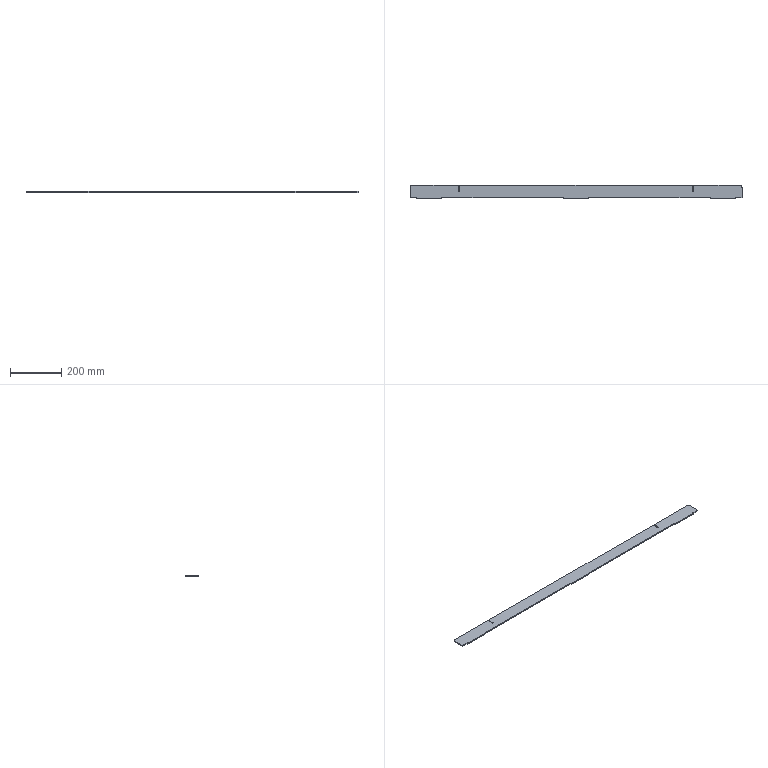Part | SolidWorks | features FlatPattern 1, SMBaseFlange 1, SheetMetal 1 | 1 solid | 28 faces | box 1300 x 54 x 4.5 mm | volume 296674 mm3 | plane 26 | cylinder 2 | commonest cylinder face diameters 20 x2
STEP:
#1=CARTESIAN_POINT('',(713.667,-1108.071,0.));
#2=VERTEX_POINT('',#1);
#3=CARTESIAN_POINT('',(713.667,-1068.071,0.));
#4=VERTEX_POINT('',#3);
#5=CARTESIAN_POINT('',(713.667,-1108.071,0.));
#6=DIRECTION('',(0.,1.,0.));
#7=VECTOR('',#6,1000.);
#8=LINE('',#5,#7);
#9=EDGE_CURVE('',#2,#4,#8,.T.);
#10=ORIENTED_EDGE('',*,*,#9,.F.);
#11=CARTESIAN_POINT('',(713.667,-1108.071,-4.5));
#12=VERTEX_POINT('',#11);
#13=CARTESIAN_POINT('',(713.667,-1108.071,-4.5));
#14=DIRECTION('',(0.,0.,1.));
#15=VECTOR('',#14,1000.);
#16=LINE('',#13,#15);
#17=EDGE_CURVE('',#12,#2,#16,.T.);
#18=ORIENTED_EDGE('',*,*,#17,.F.);
#19=CARTESIAN_POINT('',(713.667,-1068.071,-4.5));
#20=VERTEX_POINT('',#19);
#21=CARTESIAN_POINT('',(713.667,-1108.071,-4.5));
#22=DIRECTION('',(0.,1.,0.));
#23=VECTOR('',#22,1000.);
#24=LINE('',#21,#23);
#25=EDGE_CURVE('',#12,#20,#24,.T.);
#26=ORIENTED_EDGE('',*,*,#25,.T.);
#27=CARTESIAN_POINT('',(713.667,-1068.071,-4.5));
#28=DIRECTION('',(0.,0.,1.));
#29=VECTOR('',#28,1000.);
#30=LINE('',#27,#29);
#31=EDGE_CURVE('',#20,#4,#30,.T.);
#32=ORIENTED_EDGE('',*,*,#31,.T.);
#33=EDGE_LOOP('',(#10,#18,#26,#32));
#34=FACE_OUTER_BOUND('',#33,.T.);
#35=CARTESIAN_POINT('',(713.667,-1108.071,-4.5));
#36=DIRECTION('',(1.,0.,0.));
#37=DIRECTION('',(0.,0.,-1.));
#38=AXIS2_PLACEMENT_3D('',#35,#36,#37);
#39=PLANE('',#38);
#40=ADVANCED_FACE('',(#34),#39,.T.);
#41=CARTESIAN_POINT('',(688.667,-1108.071,0.));
#42=VERTEX_POINT('',#41);
#43=CARTESIAN_POINT('',(713.667,-1108.071,0.));
#44=DIRECTION('',(1.,0.,0.));
#45=VECTOR('',#44,1000.);
#46=LINE('',#43,#45);
#47=EDGE_CURVE('',#42,#2,#46,.T.);
#48=ORIENTED_EDGE('',*,*,#47,.F.);
#49=CARTESIAN_POINT('',(688.667,-1108.071,-4.5));
#50=VERTEX_POINT('',#49);
#51=CARTESIAN_POINT('',(688.667,-1108.071,-4.5));
#52=DIRECTION('',(0.,0.,1.));
#53=VECTOR('',#52,1000.);
#54=LINE('',#51,#53);
#55=EDGE_CURVE('',#50,#42,#54,.T.);
#56=ORIENTED_EDGE('',*,*,#55,.F.);
#57=CARTESIAN_POINT('',(713.667,-1108.071,-4.5));
#58=DIRECTION('',(1.,0.,0.));
#59=VECTOR('',#58,1000.);
#60=LINE('',#57,#59);
#61=EDGE_CURVE('',#50,#12,#60,.T.);
#62=ORIENTED_EDGE('',*,*,#61,.T.);
#63=ORIENTED_EDGE('',*,*,#17,.T.);
#64=EDGE_LOOP('',(#48,#56,#62,#63));
#65=FACE_OUTER_BOUND('',#64,.T.);
#66=CARTESIAN_POINT('',(713.667,-1108.071,-4.5));
#67=DIRECTION('',(0.,-1.,0.));
#68=DIRECTION('',(0.,0.,-1.));
#69=AXIS2_PLACEMENT_3D('',#66,#67,#68);
#70=PLANE('',#69);
#71=ADVANCED_FACE('',(#65),#70,.T.);
#72=CARTESIAN_POINT('',(688.667,-1112.071,0.));
#73=VERTEX_POINT('',#72);
#74=CARTESIAN_POINT('',(688.667,-1108.071,0.));
#75=DIRECTION('',(0.,1.,0.));
#76=VECTOR('',#75,1000.);
#77=LINE('',#74,#76);
#78=EDGE_CURVE('',#73,#42,#77,.T.);
#79=ORIENTED_EDGE('',*,*,#78,.F.);
#80=CARTESIAN_POINT('',(688.667,-1112.071,-4.5));
#81=VERTEX_POINT('',#80);
#82=CARTESIAN_POINT('',(688.667,-1112.071,-4.5));
#83=DIRECTION('',(0.,0.,1.));
#84=VECTOR('',#83,1000.);
#85=LINE('',#82,#84);
#86=EDGE_CURVE('',#81,#73,#85,.T.);
#87=ORIENTED_EDGE('',*,*,#86,.F.);
#88=CARTESIAN_POINT('',(688.667,-1108.071,-4.5));
#89=DIRECTION('',(0.,1.,0.));
#90=VECTOR('',#89,1000.);
#91=LINE('',#88,#90);
#92=EDGE_CURVE('',#81,#50,#91,.T.);
#93=ORIENTED_EDGE('',*,*,#92,.T.);
#94=ORIENTED_EDGE('',*,*,#55,.T.);
#95=EDGE_LOOP('',(#79,#87,#93,#94));
#96=FACE_OUTER_BOUND('',#95,.T.);
#97=CARTESIAN_POINT('',(688.667,-1108.071,-4.5));
#98=DIRECTION('',(1.,0.,0.));
#99=DIRECTION('',(0.,0.,-1.));
#100=AXIS2_PLACEMENT_3D('',#97,#98,#99);
#101=PLANE('',#100);
#102=ADVANCED_FACE('',(#96),#101,.T.);
#103=CARTESIAN_POINT('',(588.667,-1112.071,0.));
#104=VERTEX_POINT('',#103);
#105=CARTESIAN_POINT('',(688.667,-1112.071,0.));
#106=DIRECTION('',(1.,0.,0.));
#107=VECTOR('',#106,1000.);
#108=LINE('',#105,#107);
#109=EDGE_CURVE('',#104,#73,#108,.T.);
#110=ORIENTED_EDGE('',*,*,#109,.F.);
#111=CARTESIAN_POINT('',(588.667,-1112.071,-4.5));
#112=VERTEX_POINT('',#111);
#113=CARTESIAN_POINT('',(588.667,-1112.071,-4.5));
#114=DIRECTION('',(0.,0.,1.));
#115=VECTOR('',#114,1000.);
#116=LINE('',#113,#115);
#117=EDGE_CURVE('',#112,#104,#116,.T.);
#118=ORIENTED_EDGE('',*,*,#117,.F.);
#119=CARTESIAN_POINT('',(688.667,-1112.071,-4.5));
#120=DIRECTION('',(1.,0.,0.));
#121=VECTOR('',#120,1000.);
#122=LINE('',#119,#121);
#123=EDGE_CURVE('',#112,#81,#122,.T.);
#124=ORIENTED_EDGE('',*,*,#123,.T.);
#125=ORIENTED_EDGE('',*,*,#86,.T.);
#126=EDGE_LOOP('',(#110,#118,#124,#125));
#127=FACE_OUTER_BOUND('',#126,.T.);
#128=CARTESIAN_POINT('',(688.667,-1112.071,-4.5));
#129=DIRECTION('',(0.,-1.,0.));
#130=DIRECTION('',(0.,0.,-1.));
#131=AXIS2_PLACEMENT_3D('',#128,#129,#130);
#132=PLANE('',#131);
#133=ADVANCED_FACE('',(#127),#132,.T.);
#134=CARTESIAN_POINT('',(588.667,-1108.071,0.));
#135=VERTEX_POINT('',#134);
#136=CARTESIAN_POINT('',(588.667,-1112.071,0.));
#137=DIRECTION('',(0.,-1.,0.));
#138=VECTOR('',#137,1000.);
#139=LINE('',#136,#138);
#140=EDGE_CURVE('',#135,#104,#139,.T.);
#141=ORIENTED_EDGE('',*,*,#140,.F.);
#142=CARTESIAN_POINT('',(588.667,-1108.071,-4.5));
#143=VERTEX_POINT('',#142);
#144=CARTESIAN_POINT('',(588.667,-1108.071,-4.5));
#145=DIRECTION('',(0.,0.,1.));
#146=VECTOR('',#145,1000.);
#147=LINE('',#144,#146);
#148=EDGE_CURVE('',#143,#135,#147,.T.);
#149=ORIENTED_EDGE('',*,*,#148,.F.);
#150=CARTESIAN_POINT('',(588.667,-1112.071,-4.5));
#151=DIRECTION('',(0.,-1.,0.));
#152=VECTOR('',#151,1000.);
#153=LINE('',#150,#152);
#154=EDGE_CURVE('',#143,#112,#153,.T.);
#155=ORIENTED_EDGE('',*,*,#154,.T.);
#156=ORIENTED_EDGE('',*,*,#117,.T.);
#157=EDGE_LOOP('',(#141,#149,#155,#156));
#158=FACE_OUTER_BOUND('',#157,.T.);
#159=CARTESIAN_POINT('',(588.667,-1112.071,-4.5));
#160=DIRECTION('',(-1.,0.,0.));
#161=DIRECTION('',(0.,0.,1.));
#162=AXIS2_PLACEMENT_3D('',#159,#160,#161);
#163=PLANE('',#162);
#164=ADVANCED_FACE('',(#158),#163,.T.);
#165=CARTESIAN_POINT('',(113.667,-1108.071,0.));
#166=VERTEX_POINT('',#165);
#167=CARTESIAN_POINT('',(588.667,-1108.071,0.));
#168=DIRECTION('',(1.,0.,0.));
#169=VECTOR('',#168,1000.);
#170=LINE('',#167,#169);
#171=EDGE_CURVE('',#166,#135,#170,.T.);
#172=ORIENTED_EDGE('',*,*,#171,.F.);
#173=CARTESIAN_POINT('',(113.667,-1108.071,-4.5));
#174=VERTEX_POINT('',#173);
#175=CARTESIAN_POINT('',(113.667,-1108.071,-4.5));
#176=DIRECTION('',(0.,0.,1.));
#177=VECTOR('',#176,1000.);
#178=LINE('',#175,#177);
#179=EDGE_CURVE('',#174,#166,#178,.T.);
#180=ORIENTED_EDGE('',*,*,#179,.F.);
#181=CARTESIAN_POINT('',(588.667,-1108.071,-4.5));
#182=DIRECTION('',(1.,0.,0.));
#183=VECTOR('',#182,1000.);
#184=LINE('',#181,#183);
#185=EDGE_CURVE('',#174,#143,#184,.T.);
#186=ORIENTED_EDGE('',*,*,#185,.T.);
#187=ORIENTED_EDGE('',*,*,#148,.T.);
#188=EDGE_LOOP('',(#172,#180,#186,#187));
#189=FACE_OUTER_BOUND('',#188,.T.);
#190=CARTESIAN_POINT('',(588.667,-1108.071,-4.5));
#191=DIRECTION('',(0.,-1.,0.));
#192=DIRECTION('',(0.,0.,-1.));
#193=AXIS2_PLACEMENT_3D('',#190,#191,#192);
#194=PLANE('',#193);
#195=ADVANCED_FACE('',(#189),#194,.T.);
#196=CARTESIAN_POINT('',(113.667,-1112.071,0.));
#197=VERTEX_POINT('',#196);
#198=CARTESIAN_POINT('',(113.667,-1108.071,0.));
#199=DIRECTION('',(0.,1.,0.));
#200=VECTOR('',#199,1000.);
#201=LINE('',#198,#200);
#202=EDGE_CURVE('',#197,#166,#201,.T.);
#203=ORIENTED_EDGE('',*,*,#202,.F.);
#204=CARTESIAN_POINT('',(113.667,-1112.071,-4.5));
#205=VERTEX_POINT('',#204);
#206=CARTESIAN_POINT('',(113.667,-1112.071,-4.5));
#207=DIRECTION('',(0.,0.,1.));
#208=VECTOR('',#207,1000.);
#209=LINE('',#206,#208);
#210=EDGE_CURVE('',#205,#197,#209,.T.);
#211=ORIENTED_EDGE('',*,*,#210,.F.);
#212=CARTESIAN_POINT('',(113.667,-1108.071,-4.5));
#213=DIRECTION('',(0.,1.,0.));
#214=VECTOR('',#213,1000.);
#215=LINE('',#212,#214);
#216=EDGE_CURVE('',#205,#174,#215,.T.);
#217=ORIENTED_EDGE('',*,*,#216,.T.);
#218=ORIENTED_EDGE('',*,*,#179,.T.);
#219=EDGE_LOOP('',(#203,#211,#217,#218));
#220=FACE_OUTER_BOUND('',#219,.T.);
#221=CARTESIAN_POINT('',(113.667,-1108.071,-4.5));
#222=DIRECTION('',(1.,0.,0.));
#223=DIRECTION('',(0.,1.,0.));
#224=AXIS2_PLACEMENT_3D('',#221,#222,#223);
#225=PLANE('',#224);
#226=ADVANCED_FACE('',(#220),#225,.T.);
#227=CARTESIAN_POINT('',(13.667,-1112.071,0.));
#228=VERTEX_POINT('',#227);
#229=CARTESIAN_POINT('',(113.667,-1112.071,0.));
#230=DIRECTION('',(1.,0.,0.));
#231=VECTOR('',#230,1000.);
#232=LINE('',#229,#231);
#233=EDGE_CURVE('',#228,#197,#232,.T.);
#234=ORIENTED_EDGE('',*,*,#233,.F.);
#235=CARTESIAN_POINT('',(13.667,-1112.071,-4.5));
#236=VERTEX_POINT('',#235);
#237=CARTESIAN_POINT('',(13.667,-1112.071,-4.5));
#238=DIRECTION('',(0.,0.,1.));
#239=VECTOR('',#238,1000.);
#240=LINE('',#237,#239);
#241=EDGE_CURVE('',#236,#228,#240,.T.);
#242=ORIENTED_EDGE('',*,*,#241,.F.);
#243=CARTESIAN_POINT('',(113.667,-1112.071,-4.5));
#244=DIRECTION('',(1.,0.,0.));
#245=VECTOR('',#244,1000.);
#246=LINE('',#243,#245);
#247=EDGE_CURVE('',#236,#205,#246,.T.);
#248=ORIENTED_EDGE('',*,*,#247,.T.);
#249=ORIENTED_EDGE('',*,*,#210,.T.);
#250=EDGE_LOOP('',(#234,#242,#248,#249));
#251=FACE_OUTER_BOUND('',#250,.T.);
#252=CARTESIAN_POINT('',(113.667,-1112.071,-4.5));
#253=DIRECTION('',(0.,-1.,0.));
#254=DIRECTION('',(0.,0.,-1.));
#255=AXIS2_PLACEMENT_3D('',#252,#253,#254);
#256=PLANE('',#255);
#257=ADVANCED_FACE('',(#251),#256,.T.);
#258=CARTESIAN_POINT('',(13.667,-1108.071,0.));
#259=VERTEX_POINT('',#258);
#260=CARTESIAN_POINT('',(13.667,-1112.071,0.));
#261=DIRECTION('',(0.,-1.,0.));
#262=VECTOR('',#261,1000.);
#263=LINE('',#260,#262);
#264=EDGE_CURVE('',#259,#228,#263,.T.);
#265=ORIENTED_EDGE('',*,*,#264,.F.);
#266=CARTESIAN_POINT('',(13.667,-1108.071,-4.5));
#267=VERTEX_POINT('',#266);
#268=CARTESIAN_POINT('',(13.667,-1108.071,-4.5));
#269=DIRECTION('',(0.,0.,1.));
#270=VECTOR('',#269,1000.);
#271=LINE('',#268,#270);
#272=EDGE_CURVE('',#267,#259,#271,.T.);
#273=ORIENTED_EDGE('',*,*,#272,.F.);
#274=CARTESIAN_POINT('',(13.667,-1112.071,-4.5));
#275=DIRECTION('',(0.,-1.,0.));
#276=VECTOR('',#275,1000.);
#277=LINE('',#274,#276);
#278=EDGE_CURVE('',#267,#236,#277,.T.);
#279=ORIENTED_EDGE('',*,*,#278,.T.);
#280=ORIENTED_EDGE('',*,*,#241,.T.);
#281=EDGE_LOOP('',(#265,#273,#279,#280));
#282=FACE_OUTER_BOUND('',#281,.T.);
#283=CARTESIAN_POINT('',(13.667,-1112.071,-4.5));
#284=DIRECTION('',(-1.,0.,0.));
#285=DIRECTION('',(0.,-1.,0.));
#286=AXIS2_PLACEMENT_3D('',#283,#284,#285);
#287=PLANE('',#286);
#288=ADVANCED_FACE('',(#282),#287,.T.);
#289=CARTESIAN_POINT('',(-461.333,-1108.071,0.));
#290=VERTEX_POINT('',#289);
#291=CARTESIAN_POINT('',(13.667,-1108.071,0.));
#292=DIRECTION('',(1.,0.,0.));
#293=VECTOR('',#292,1000.);
#294=LINE('',#291,#293);
#295=EDGE_CURVE('',#290,#259,#294,.T.);
#296=ORIENTED_EDGE('',*,*,#295,.F.);
#297=CARTESIAN_POINT('',(-461.333,-1108.071,-4.5));
#298=VERTEX_POINT('',#297);
#299=CARTESIAN_POINT('',(-461.333,-1108.071,-4.5));
#300=DIRECTION('',(0.,0.,1.));
#301=VECTOR('',#300,1000.);
#302=LINE('',#299,#301);
#303=EDGE_CURVE('',#298,#290,#302,.T.);
#304=ORIENTED_EDGE('',*,*,#303,.F.);
#305=CARTESIAN_POINT('',(13.667,-1108.071,-4.5));
#306=DIRECTION('',(1.,0.,0.));
#307=VECTOR('',#306,1000.);
#308=LINE('',#305,#307);
#309=EDGE_CURVE('',#298,#267,#308,.T.);
#310=ORIENTED_EDGE('',*,*,#309,.T.);
#311=ORIENTED_EDGE('',*,*,#272,.T.);
#312=EDGE_LOOP('',(#296,#304,#310,#311));
#313=FACE_OUTER_BOUND('',#312,.T.);
#314=CARTESIAN_POINT('',(13.667,-1108.071,-4.5));
#315=DIRECTION('',(0.,-1.,0.));
#316=DIRECTION('',(0.,0.,-1.));
#317=AXIS2_PLACEMENT_3D('',#314,#315,#316);
#318=PLANE('',#317);
#319=ADVANCED_FACE('',(#313),#318,.T.);
#320=CARTESIAN_POINT('',(-461.333,-1112.071,0.));
#321=VERTEX_POINT('',#320);
#322=CARTESIAN_POINT('',(-461.333,-1112.071,0.));
#323=DIRECTION('',(0.,1.,0.));
#324=VECTOR('',#323,1000.);
#325=LINE('',#322,#324);
#326=EDGE_CURVE('',#321,#290,#325,.T.);
#327=ORIENTED_EDGE('',*,*,#326,.F.);
#328=CARTESIAN_POINT('',(-461.333,-1112.071,-4.5));
#329=VERTEX_POINT('',#328);
#330=CARTESIAN_POINT('',(-461.333,-1112.071,-4.5));
#331=DIRECTION('',(0.,0.,1.));
#332=VECTOR('',#331,1000.);
#333=LINE('',#330,#332);
#334=EDGE_CURVE('',#329,#321,#333,.T.);
#335=ORIENTED_EDGE('',*,*,#334,.F.);
#336=CARTESIAN_POINT('',(-461.333,-1112.071,-4.5));
#337=DIRECTION('',(0.,1.,0.));
#338=VECTOR('',#337,1000.);
#339=LINE('',#336,#338);
#340=EDGE_CURVE('',#329,#298,#339,.T.);
#341=ORIENTED_EDGE('',*,*,#340,.T.);
#342=ORIENTED_EDGE('',*,*,#303,.T.);
#343=EDGE_LOOP('',(#327,#335,#341,#342));
#344=FACE_OUTER_BOUND('',#343,.T.);
#345=CARTESIAN_POINT('',(-461.333,-1112.071,-4.5));
#346=DIRECTION('',(1.,0.,0.));
#347=DIRECTION('',(0.,0.,-1.));
#348=AXIS2_PLACEMENT_3D('',#345,#346,#347);
#349=PLANE('',#348);
#350=ADVANCED_FACE('',(#344),#349,.T.);
#351=CARTESIAN_POINT('',(-561.333,-1112.071,0.));
#352=VERTEX_POINT('',#351);
#353=CARTESIAN_POINT('',(-561.333,-1112.071,0.));
#354=DIRECTION('',(1.,0.,0.));
#355=VECTOR('',#354,1000.);
#356=LINE('',#353,#355);
#357=EDGE_CURVE('',#352,#321,#356,.T.);
#358=ORIENTED_EDGE('',*,*,#357,.F.);
#359=CARTESIAN_POINT('',(-561.333,-1112.071,-4.5));
#360=VERTEX_POINT('',#359);
#361=CARTESIAN_POINT('',(-561.333,-1112.071,-4.5));
#362=DIRECTION('',(0.,0.,1.));
#363=VECTOR('',#362,1000.);
#364=LINE('',#361,#363);
#365=EDGE_CURVE('',#360,#352,#364,.T.);
#366=ORIENTED_EDGE('',*,*,#365,.F.);
#367=CARTESIAN_POINT('',(-561.333,-1112.071,-4.5));
#368=DIRECTION('',(1.,0.,0.));
#369=VECTOR('',#368,1000.);
#370=LINE('',#367,#369);
#371=EDGE_CURVE('',#360,#329,#370,.T.);
#372=ORIENTED_EDGE('',*,*,#371,.T.);
#373=ORIENTED_EDGE('',*,*,#334,.T.);
#374=EDGE_LOOP('',(#358,#366,#372,#373));
#375=FACE_OUTER_BOUND('',#374,.T.);
#376=CARTESIAN_POINT('',(-561.333,-1112.071,-4.5));
#377=DIRECTION('',(0.,-1.,0.));
#378=DIRECTION('',(0.,0.,-1.));
#379=AXIS2_PLACEMENT_3D('',#376,#377,#378);
#380=PLANE('',#379);
#381=ADVANCED_FACE('',(#375),#380,.T.);
#382=CARTESIAN_POINT('',(-561.333,-1108.071,0.));
#383=VERTEX_POINT('',#382);
#384=CARTESIAN_POINT('',(-561.333,-1108.071,0.));
#385=DIRECTION('',(0.,-1.,0.));
#386=VECTOR('',#385,1000.);
#387=LINE('',#384,#386);
#388=EDGE_CURVE('',#383,#352,#387,.T.);
#389=ORIENTED_EDGE('',*,*,#388,.F.);
#390=CARTESIAN_POINT('',(-561.333,-1108.071,-4.5));
#391=VERTEX_POINT('',#390);
#392=CARTESIAN_POINT('',(-561.333,-1108.071,-4.5));
#393=DIRECTION('',(0.,0.,1.));
#394=VECTOR('',#393,1000.);
#395=LINE('',#392,#394);
#396=EDGE_CURVE('',#391,#383,#395,.T.);
#397=ORIENTED_EDGE('',*,*,#396,.F.);
#398=CARTESIAN_POINT('',(-561.333,-1108.071,-4.5));
#399=DIRECTION('',(0.,-1.,0.));
#400=VECTOR('',#399,1000.);
#401=LINE('',#398,#400);
#402=EDGE_CURVE('',#391,#360,#401,.T.);
#403=ORIENTED_EDGE('',*,*,#402,.T.);
#404=ORIENTED_EDGE('',*,*,#365,.T.);
#405=EDGE_LOOP('',(#389,#397,#403,#404));
#406=FACE_OUTER_BOUND('',#405,.T.);
#407=CARTESIAN_POINT('',(-561.333,-1108.071,-4.5));
#408=DIRECTION('',(-1.,0.,0.));
#409=DIRECTION('',(0.,0.,1.));
#410=AXIS2_PLACEMENT_3D('',#407,#408,#409);
#411=PLANE('',#410);
#412=ADVANCED_FACE('',(#406),#411,.T.);
#413=CARTESIAN_POINT('',(-586.333,-1108.071,0.));
#414=VERTEX_POINT('',#413);
#415=CARTESIAN_POINT('',(-561.333,-1108.071,0.));
#416=DIRECTION('',(1.,0.,0.));
#417=VECTOR('',#416,1000.);
#418=LINE('',#415,#417);
#419=EDGE_CURVE('',#414,#383,#418,.T.);
#420=ORIENTED_EDGE('',*,*,#419,.F.);
#421=CARTESIAN_POINT('',(-586.333,-1108.071,-4.5));
#422=VERTEX_POINT('',#421);
#423=CARTESIAN_POINT('',(-586.333,-1108.071,-4.5));
#424=DIRECTION('',(0.,0.,1.));
#425=VECTOR('',#424,1000.);
#426=LINE('',#423,#425);
#427=EDGE_CURVE('',#422,#414,#426,.T.);
#428=ORIENTED_EDGE('',*,*,#427,.F.);
#429=CARTESIAN_POINT('',(-561.333,-1108.071,-4.5));
#430=DIRECTION('',(1.,0.,0.));
#431=VECTOR('',#430,1000.);
#432=LINE('',#429,#431);
#433=EDGE_CURVE('',#422,#391,#432,.T.);
#434=ORIENTED_EDGE('',*,*,#433,.T.);
#435=ORIENTED_EDGE('',*,*,#396,.T.);
#436=EDGE_LOOP('',(#420,#428,#434,#435));
#437=FACE_OUTER_BOUND('',#436,.T.);
#438=CARTESIAN_POINT('',(-561.333,-1108.071,-4.5));
#439=DIRECTION('',(0.,-1.,0.));
#440=DIRECTION('',(0.,0.,-1.));
#441=AXIS2_PLACEMENT_3D('',#438,#439,#440);
#442=PLANE('',#441);
#443=ADVANCED_FACE('',(#437),#442,.T.);
#444=CARTESIAN_POINT('',(-586.333,-1068.071,0.));
#445=VERTEX_POINT('',#444);
#446=CARTESIAN_POINT('',(-586.333,-1108.071,0.));
#447=DIRECTION('',(0.,-1.,0.));
#448=VECTOR('',#447,1000.);
#449=LINE('',#446,#448);
#450=EDGE_CURVE('',#445,#414,#449,.T.);
#451=ORIENTED_EDGE('',*,*,#450,.F.);
#452=CARTESIAN_POINT('',(-586.333,-1068.071,-4.5));
#453=VERTEX_POINT('',#452);
#454=CARTESIAN_POINT('',(-586.333,-1068.071,-4.5));
#455=DIRECTION('',(0.,0.,1.));
#456=VECTOR('',#455,1000.);
#457=LINE('',#454,#456);
#458=EDGE_CURVE('',#453,#445,#457,.T.);
#459=ORIENTED_EDGE('',*,*,#458,.F.);
#460=CARTESIAN_POINT('',(-586.333,-1108.071,-4.5));
#461=DIRECTION('',(0.,-1.,0.));
#462=VECTOR('',#461,1000.);
#463=LINE('',#460,#462);
#464=EDGE_CURVE('',#453,#422,#463,.T.);
#465=ORIENTED_EDGE('',*,*,#464,.T.);
#466=ORIENTED_EDGE('',*,*,#427,.T.);
#467=EDGE_LOOP('',(#451,#459,#465,#466));
#468=FACE_OUTER_BOUND('',#467,.T.);
#469=CARTESIAN_POINT('',(-586.333,-1108.071,-4.5));
#470=DIRECTION('',(-1.,0.,0.));
#471=DIRECTION('',(0.,0.,1.));
#472=AXIS2_PLACEMENT_3D('',#469,#470,#471);
#473=PLANE('',#472);
#474=ADVANCED_FACE('',(#468),#473,.T.);
#475=CARTESIAN_POINT('',(-576.333,-1058.071,0.));
#476=VERTEX_POINT('',#475);
#477=CARTESIAN_POINT('',(-576.333,-1068.071,0.));
#478=DIRECTION('',(0.,0.,1.));
#479=DIRECTION('',(1.,0.,0.));
#480=AXIS2_PLACEMENT_3D('',#477,#478,#479);
#481=CIRCLE('',#480,10.);
#482=EDGE_CURVE('',#476,#445,#481,.T.);
#483=ORIENTED_EDGE('',*,*,#482,.F.);
#484=CARTESIAN_POINT('',(-576.333,-1058.071,-4.5));
#485=VERTEX_POINT('',#484);
#486=CARTESIAN_POINT('',(-576.333,-1058.071,-4.5));
#487=DIRECTION('',(0.,0.,1.));
#488=VECTOR('',#487,1000.);
#489=LINE('',#486,#488);
#490=EDGE_CURVE('',#485,#476,#489,.T.);
#491=ORIENTED_EDGE('',*,*,#490,.F.);
#492=CARTESIAN_POINT('',(-576.333,-1068.071,-4.5));
#493=DIRECTION('',(0.,0.,1.));
#494=DIRECTION('',(1.,0.,0.));
#495=AXIS2_PLACEMENT_3D('',#492,#493,#494);
#496=CIRCLE('',#495,10.);
#497=EDGE_CURVE('',#485,#453,#496,.T.);
#498=ORIENTED_EDGE('',*,*,#497,.T.);
#499=ORIENTED_EDGE('',*,*,#458,.T.);
#500=EDGE_LOOP('',(#483,#491,#498,#499));
#501=FACE_OUTER_BOUND('',#500,.T.);
#502=CARTESIAN_POINT('',(-576.333,-1068.071,-4.5));
#503=DIRECTION('',(0.,0.,1.));
#504=DIRECTION('',(1.,0.,0.));
#505=AXIS2_PLACEMENT_3D('',#502,#503,#504);
#506=CYLINDRICAL_SURFACE('',#505,10.);
#507=ADVANCED_FACE('',(#501),#506,.T.);
#508=CARTESIAN_POINT('',(-396.333,-1058.071,0.));
#509=VERTEX_POINT('',#508);
#510=CARTESIAN_POINT('',(-396.333,-1058.071,0.));
#511=DIRECTION('',(-1.,0.,0.));
#512=VECTOR('',#511,1000.);
#513=LINE('',#510,#512);
#514=EDGE_CURVE('',#509,#476,#513,.T.);
#515=ORIENTED_EDGE('',*,*,#514,.F.);
#516=CARTESIAN_POINT('',(-396.333,-1058.071,-4.5));
#517=VERTEX_POINT('',#516);
#518=CARTESIAN_POINT('',(-396.333,-1058.071,-4.5));
#519=DIRECTION('',(0.,0.,1.));
#520=VECTOR('',#519,1000.);
#521=LINE('',#518,#520);
#522=EDGE_CURVE('',#517,#509,#521,.T.);
#523=ORIENTED_EDGE('',*,*,#522,.F.);
#524=CARTESIAN_POINT('',(-396.333,-1058.071,-4.5));
#525=DIRECTION('',(-1.,0.,0.));
#526=VECTOR('',#525,1000.);
#527=LINE('',#524,#526);
#528=EDGE_CURVE('',#517,#485,#527,.T.);
#529=ORIENTED_EDGE('',*,*,#528,.T.);
#530=ORIENTED_EDGE('',*,*,#490,.T.);
#531=EDGE_LOOP('',(#515,#523,#529,#530));
#532=FACE_OUTER_BOUND('',#531,.T.);
#533=CARTESIAN_POINT('',(-396.333,-1058.071,-4.5));
#534=DIRECTION('',(0.,1.,0.));
#535=DIRECTION('',(0.,0.,1.));
#536=AXIS2_PLACEMENT_3D('',#533,#534,#535);
#537=PLANE('',#536);
#538=ADVANCED_FACE('',(#532),#537,.T.);
#539=CARTESIAN_POINT('',(-396.333,-1083.571,0.));
#540=VERTEX_POINT('',#539);
#541=CARTESIAN_POINT('',(-396.333,-1083.571,0.));
#542=DIRECTION('',(0.,1.,0.));
#543=VECTOR('',#542,1000.);
#544=LINE('',#541,#543);
#545=EDGE_CURVE('',#540,#509,#544,.T.);
#546=ORIENTED_EDGE('',*,*,#545,.F.);
#547=CARTESIAN_POINT('',(-396.333,-1083.571,-4.5));
#548=VERTEX_POINT('',#547);
#549=CARTESIAN_POINT('',(-396.333,-1083.571,-4.5));
#550=DIRECTION('',(0.,0.,1.));
#551=VECTOR('',#550,1000.);
#552=LINE('',#549,#551);
#553=EDGE_CURVE('',#548,#540,#552,.T.);
#554=ORIENTED_EDGE('',*,*,#553,.F.);
#555=CARTESIAN_POINT('',(-396.333,-1083.571,-4.5));
#556=DIRECTION('',(0.,1.,0.));
#557=VECTOR('',#556,1000.);
#558=LINE('',#555,#557);
#559=EDGE_CURVE('',#548,#517,#558,.T.);
#560=ORIENTED_EDGE('',*,*,#559,.T.);
#561=ORIENTED_EDGE('',*,*,#522,.T.);
#562=EDGE_LOOP('',(#546,#554,#560,#561));
#563=FACE_OUTER_BOUND('',#562,.T.);
#564=CARTESIAN_POINT('',(-396.333,-1083.571,-4.5));
#565=DIRECTION('',(1.,0.,0.));
#566=DIRECTION('',(0.,0.,-1.));
#567=AXIS2_PLACEMENT_3D('',#564,#565,#566);
#568=PLANE('',#567);
#569=ADVANCED_FACE('',(#563),#568,.T.);
#570=CARTESIAN_POINT('',(-391.833,-1083.571,0.));
#571=VERTEX_POINT('',#570);
#572=CARTESIAN_POINT('',(-391.833,-1083.571,0.));
#573=DIRECTION('',(-1.,0.,0.));
#574=VECTOR('',#573,1000.);
#575=LINE('',#572,#574);
#576=EDGE_CURVE('',#571,#540,#575,.T.);
#577=ORIENTED_EDGE('',*,*,#576,.F.);
#578=CARTESIAN_POINT('',(-391.833,-1083.571,-4.5));
#579=VERTEX_POINT('',#578);
#580=CARTESIAN_POINT('',(-391.833,-1083.571,-4.5));
#581=DIRECTION('',(0.,0.,1.));
#582=VECTOR('',#581,1000.);
#583=LINE('',#580,#582);
#584=EDGE_CURVE('',#579,#571,#583,.T.);
#585=ORIENTED_EDGE('',*,*,#584,.F.);
#586=CARTESIAN_POINT('',(-391.833,-1083.571,-4.5));
#587=DIRECTION('',(-1.,0.,0.));
#588=VECTOR('',#587,1000.);
#589=LINE('',#586,#588);
#590=EDGE_CURVE('',#579,#548,#589,.T.);
#591=ORIENTED_EDGE('',*,*,#590,.T.);
#592=ORIENTED_EDGE('',*,*,#553,.T.);
#593=EDGE_LOOP('',(#577,#585,#591,#592));
#594=FACE_OUTER_BOUND('',#593,.T.);
#595=CARTESIAN_POINT('',(-391.833,-1083.571,-4.5));
#596=DIRECTION('',(0.,1.,0.));
#597=DIRECTION('',(0.,0.,1.));
#598=AXIS2_PLACEMENT_3D('',#595,#596,#597);
#599=PLANE('',#598);
#600=ADVANCED_FACE('',(#594),#599,.T.);
#601=CARTESIAN_POINT('',(-391.833,-1058.071,0.));
#602=VERTEX_POINT('',#601);
#603=CARTESIAN_POINT('',(-391.833,-1058.071,0.));
#604=DIRECTION('',(0.,-1.,0.));
#605=VECTOR('',#604,1000.);
#606=LINE('',#603,#605);
#607=EDGE_CURVE('',#602,#571,#606,.T.);
#608=ORIENTED_EDGE('',*,*,#607,.F.);
#609=CARTESIAN_POINT('',(-391.833,-1058.071,-4.5));
#610=VERTEX_POINT('',#609);
#611=CARTESIAN_POINT('',(-391.833,-1058.071,-4.5));
#612=DIRECTION('',(0.,0.,1.));
#613=VECTOR('',#612,1000.);
#614=LINE('',#611,#613);
#615=EDGE_CURVE('',#610,#602,#614,.T.);
#616=ORIENTED_EDGE('',*,*,#615,.F.);
#617=CARTESIAN_POINT('',(-391.833,-1058.071,-4.5));
#618=DIRECTION('',(0.,-1.,0.));
#619=VECTOR('',#618,1000.);
#620=LINE('',#617,#619);
#621=EDGE_CURVE('',#610,#579,#620,.T.);
#622=ORIENTED_EDGE('',*,*,#621,.T.);
#623=ORIENTED_EDGE('',*,*,#584,.T.);
#624=EDGE_LOOP('',(#608,#616,#622,#623));
#625=FACE_OUTER_BOUND('',#624,.T.);
#626=CARTESIAN_POINT('',(-391.833,-1058.071,-4.5));
#627=DIRECTION('',(-1.,0.,0.));
#628=DIRECTION('',(0.,0.,1.));
#629=AXIS2_PLACEMENT_3D('',#626,#627,#628);
#630=PLANE('',#629);
#631=ADVANCED_FACE('',(#625),#630,.T.);
#632=CARTESIAN_POINT('',(519.167,-1058.071,0.));
#633=VERTEX_POINT('',#632);
#634=CARTESIAN_POINT('',(519.167,-1058.071,0.));
#635=DIRECTION('',(-1.,0.,0.));
#636=VECTOR('',#635,1000.);
#637=LINE('',#634,#636);
#638=EDGE_CURVE('',#633,#602,#637,.T.);
#639=ORIENTED_EDGE('',*,*,#638,.F.);
#640=CARTESIAN_POINT('',(519.167,-1058.071,-4.5));
#641=VERTEX_POINT('',#640);
#642=CARTESIAN_POINT('',(519.167,-1058.071,-4.5));
#643=DIRECTION('',(0.,0.,1.));
#644=VECTOR('',#643,1000.);
#645=LINE('',#642,#644);
#646=EDGE_CURVE('',#641,#633,#645,.T.);
#647=ORIENTED_EDGE('',*,*,#646,.F.);
#648=CARTESIAN_POINT('',(519.167,-1058.071,-4.5));
#649=DIRECTION('',(-1.,0.,0.));
#650=VECTOR('',#649,1000.);
#651=LINE('',#648,#650);
#652=EDGE_CURVE('',#641,#610,#651,.T.);
#653=ORIENTED_EDGE('',*,*,#652,.T.);
#654=ORIENTED_EDGE('',*,*,#615,.T.);
#655=EDGE_LOOP('',(#639,#647,#653,#654));
#656=FACE_OUTER_BOUND('',#655,.T.);
#657=CARTESIAN_POINT('',(519.167,-1058.071,-4.5));
#658=DIRECTION('',(0.,1.,0.));
#659=DIRECTION('',(0.,0.,1.));
#660=AXIS2_PLACEMENT_3D('',#657,#658,#659);
#661=PLANE('',#660);
#662=ADVANCED_FACE('',(#656),#661,.T.);
#663=CARTESIAN_POINT('',(519.167,-1083.571,0.));
#664=VERTEX_POINT('',#663);
#665=CARTESIAN_POINT('',(519.167,-1083.571,0.));
#666=DIRECTION('',(0.,1.,0.));
#667=VECTOR('',#666,1000.);
#668=LINE('',#665,#667);
#669=EDGE_CURVE('',#664,#633,#668,.T.);
#670=ORIENTED_EDGE('',*,*,#669,.F.);
#671=CARTESIAN_POINT('',(519.167,-1083.571,-4.5));
#672=VERTEX_POINT('',#671);
#673=CARTESIAN_POINT('',(519.167,-1083.571,-4.5));
#674=DIRECTION('',(0.,0.,1.));
#675=VECTOR('',#674,1000.);
#676=LINE('',#673,#675);
#677=EDGE_CURVE('',#672,#664,#676,.T.);
#678=ORIENTED_EDGE('',*,*,#677,.F.);
#679=CARTESIAN_POINT('',(519.167,-1083.571,-4.5));
#680=DIRECTION('',(0.,1.,0.));
#681=VECTOR('',#680,1000.);
#682=LINE('',#679,#681);
#683=EDGE_CURVE('',#672,#641,#682,.T.);
#684=ORIENTED_EDGE('',*,*,#683,.T.);
#685=ORIENTED_EDGE('',*,*,#646,.T.);
#686=EDGE_LOOP('',(#670,#678,#684,#685));
#687=FACE_OUTER_BOUND('',#686,.T.);
#688=CARTESIAN_POINT('',(519.167,-1083.571,-4.5));
#689=DIRECTION('',(1.,0.,0.));
#690=DIRECTION('',(0.,0.,-1.));
#691=AXIS2_PLACEMENT_3D('',#688,#689,#690);
#692=PLANE('',#691);
#693=ADVANCED_FACE('',(#687),#692,.T.);
#694=CARTESIAN_POINT('',(523.667,-1083.571,0.));
#695=VERTEX_POINT('',#694);
#696=CARTESIAN_POINT('',(523.667,-1083.571,0.));
#697=DIRECTION('',(-1.,0.,0.));
#698=VECTOR('',#697,1000.);
#699=LINE('',#696,#698);
#700=EDGE_CURVE('',#695,#664,#699,.T.);
#701=ORIENTED_EDGE('',*,*,#700,.F.);
#702=CARTESIAN_POINT('',(523.667,-1083.571,-4.5));
#703=VERTEX_POINT('',#702);
#704=CARTESIAN_POINT('',(523.667,-1083.571,-4.5));
#705=DIRECTION('',(0.,0.,1.));
#706=VECTOR('',#705,1000.);
#707=LINE('',#704,#706);
#708=EDGE_CURVE('',#703,#695,#707,.T.);
#709=ORIENTED_EDGE('',*,*,#708,.F.);
#710=CARTESIAN_POINT('',(523.667,-1083.571,-4.5));
#711=DIRECTION('',(-1.,0.,0.));
#712=VECTOR('',#711,1000.);
#713=LINE('',#710,#712);
#714=EDGE_CURVE('',#703,#672,#713,.T.);
#715=ORIENTED_EDGE('',*,*,#714,.T.);
#716=ORIENTED_EDGE('',*,*,#677,.T.);
#717=EDGE_LOOP('',(#701,#709,#715,#716));
#718=FACE_OUTER_BOUND('',#717,.T.);
#719=CARTESIAN_POINT('',(523.667,-1083.571,-4.5));
#720=DIRECTION('',(0.,1.,0.));
#721=DIRECTION('',(0.,0.,1.));
#722=AXIS2_PLACEMENT_3D('',#719,#720,#721);
#723=PLANE('',#722);
#724=ADVANCED_FACE('',(#718),#723,.T.);
#725=CARTESIAN_POINT('',(523.667,-1058.071,0.));
#726=VERTEX_POINT('',#725);
#727=CARTESIAN_POINT('',(523.667,-1058.071,0.));
#728=DIRECTION('',(0.,-1.,0.));
#729=VECTOR('',#728,1000.);
#730=LINE('',#727,#729);
#731=EDGE_CURVE('',#726,#695,#730,.T.);
#732=ORIENTED_EDGE('',*,*,#731,.F.);
#733=CARTESIAN_POINT('',(523.667,-1058.071,-4.5));
#734=VERTEX_POINT('',#733);
#735=CARTESIAN_POINT('',(523.667,-1058.071,-4.5));
#736=DIRECTION('',(0.,0.,1.));
#737=VECTOR('',#736,1000.);
#738=LINE('',#735,#737);
#739=EDGE_CURVE('',#734,#726,#738,.T.);
#740=ORIENTED_EDGE('',*,*,#739,.F.);
#741=CARTESIAN_POINT('',(523.667,-1058.071,-4.5));
#742=DIRECTION('',(0.,-1.,0.));
#743=VECTOR('',#742,1000.);
#744=LINE('',#741,#743);
#745=EDGE_CURVE('',#734,#703,#744,.T.);
#746=ORIENTED_EDGE('',*,*,#745,.T.);
#747=ORIENTED_EDGE('',*,*,#708,.T.);
#748=EDGE_LOOP('',(#732,#740,#746,#747));
#749=FACE_OUTER_BOUND('',#748,.T.);
#750=CARTESIAN_POINT('',(523.667,-1058.071,-4.5));
#751=DIRECTION('',(-1.,0.,0.));
#752=DIRECTION('',(0.,0.,1.));
#753=AXIS2_PLACEMENT_3D('',#750,#751,#752);
#754=PLANE('',#753);
#755=ADVANCED_FACE('',(#749),#754,.T.);
#756=CARTESIAN_POINT('',(703.667,-1058.071,0.));
#757=VERTEX_POINT('',#756);
#758=CARTESIAN_POINT('',(703.667,-1058.071,0.));
#759=DIRECTION('',(-1.,0.,0.));
#760=VECTOR('',#759,1000.);
#761=LINE('',#758,#760);
#762=EDGE_CURVE('',#757,#726,#761,.T.);
#763=ORIENTED_EDGE('',*,*,#762,.F.);
#764=CARTESIAN_POINT('',(703.667,-1058.071,-4.5));
#765=VERTEX_POINT('',#764);
#766=CARTESIAN_POINT('',(703.667,-1058.071,-4.5));
#767=DIRECTION('',(0.,0.,1.));
#768=VECTOR('',#767,1000.);
#769=LINE('',#766,#768);
#770=EDGE_CURVE('',#765,#757,#769,.T.);
#771=ORIENTED_EDGE('',*,*,#770,.F.);
#772=CARTESIAN_POINT('',(703.667,-1058.071,-4.5));
#773=DIRECTION('',(-1.,0.,0.));
#774=VECTOR('',#773,1000.);
#775=LINE('',#772,#774);
#776=EDGE_CURVE('',#765,#734,#775,.T.);
#777=ORIENTED_EDGE('',*,*,#776,.T.);
#778=ORIENTED_EDGE('',*,*,#739,.T.);
#779=EDGE_LOOP('',(#763,#771,#777,#778));
#780=FACE_OUTER_BOUND('',#779,.T.);
#781=CARTESIAN_POINT('',(703.667,-1058.071,-4.5));
#782=DIRECTION('',(0.,1.,0.));
#783=DIRECTION('',(0.,0.,1.));
#784=AXIS2_PLACEMENT_3D('',#781,#782,#783);
#785=PLANE('',#784);
#786=ADVANCED_FACE('',(#780),#785,.T.);
#787=CARTESIAN_POINT('',(703.667,-1068.071,0.));
#788=DIRECTION('',(0.,0.,1.));
#789=DIRECTION('',(1.,0.,0.));
#790=AXIS2_PLACEMENT_3D('',#787,#788,#789);
#791=CIRCLE('',#790,10.);
#792=EDGE_CURVE('',#4,#757,#791,.T.);
#793=ORIENTED_EDGE('',*,*,#792,.F.);
#794=ORIENTED_EDGE('',*,*,#31,.F.);
#795=CARTESIAN_POINT('',(703.667,-1068.071,-4.5));
#796=DIRECTION('',(0.,0.,1.));
#797=DIRECTION('',(1.,0.,0.));
#798=AXIS2_PLACEMENT_3D('',#795,#796,#797);
#799=CIRCLE('',#798,10.);
#800=EDGE_CURVE('',#20,#765,#799,.T.);
#801=ORIENTED_EDGE('',*,*,#800,.T.);
#802=ORIENTED_EDGE('',*,*,#770,.T.);
#803=EDGE_LOOP('',(#793,#794,#801,#802));
#804=FACE_OUTER_BOUND('',#803,.T.);
#805=CARTESIAN_POINT('',(703.667,-1068.071,-4.5));
#806=DIRECTION('',(0.,0.,1.));
#807=DIRECTION('',(1.,0.,0.));
#808=AXIS2_PLACEMENT_3D('',#805,#806,#807);
#809=CYLINDRICAL_SURFACE('',#808,10.);
#810=ADVANCED_FACE('',(#804),#809,.T.);
#811=ORIENTED_EDGE('',*,*,#25,.F.);
#812=ORIENTED_EDGE('',*,*,#61,.F.);
#813=ORIENTED_EDGE('',*,*,#92,.F.);
#814=ORIENTED_EDGE('',*,*,#123,.F.);
#815=ORIENTED_EDGE('',*,*,#154,.F.);
#816=ORIENTED_EDGE('',*,*,#185,.F.);
#817=ORIENTED_EDGE('',*,*,#216,.F.);
#818=ORIENTED_EDGE('',*,*,#247,.F.);
#819=ORIENTED_EDGE('',*,*,#278,.F.);
#820=ORIENTED_EDGE('',*,*,#309,.F.);
#821=ORIENTED_EDGE('',*,*,#340,.F.);
#822=ORIENTED_EDGE('',*,*,#371,.F.);
#823=ORIENTED_EDGE('',*,*,#402,.F.);
#824=ORIENTED_EDGE('',*,*,#433,.F.);
#825=ORIENTED_EDGE('',*,*,#464,.F.);
#826=ORIENTED_EDGE('',*,*,#497,.F.);
#827=ORIENTED_EDGE('',*,*,#528,.F.);
#828=ORIENTED_EDGE('',*,*,#559,.F.);
#829=ORIENTED_EDGE('',*,*,#590,.F.);
#830=ORIENTED_EDGE('',*,*,#621,.F.);
#831=ORIENTED_EDGE('',*,*,#652,.F.);
#832=ORIENTED_EDGE('',*,*,#683,.F.);
#833=ORIENTED_EDGE('',*,*,#714,.F.);
#834=ORIENTED_EDGE('',*,*,#745,.F.);
#835=ORIENTED_EDGE('',*,*,#776,.F.);
#836=ORIENTED_EDGE('',*,*,#800,.F.);
#837=EDGE_LOOP('',(#811,#812,#813,#814,#815,#816,#817,#818,#819,#820,#821,#822,#823,#824,#825,#826,#827,#828,#829,#830,#831,#832,#833,#834,#835,#836));
#838=FACE_OUTER_BOUND('',#837,.T.);
#839=CARTESIAN_POINT('',(703.667,-1068.071,-4.5));
#840=DIRECTION('',(0.,0.,1.));
#841=DIRECTION('',(1.,0.,0.));
#842=AXIS2_PLACEMENT_3D('',#839,#840,#841);
#843=PLANE('',#842);
#844=ADVANCED_FACE('',(#838),#843,.F.);
#845=ORIENTED_EDGE('',*,*,#9,.T.);
#846=ORIENTED_EDGE('',*,*,#792,.T.);
#847=ORIENTED_EDGE('',*,*,#762,.T.);
#848=ORIENTED_EDGE('',*,*,#731,.T.);
#849=ORIENTED_EDGE('',*,*,#700,.T.);
#850=ORIENTED_EDGE('',*,*,#669,.T.);
#851=ORIENTED_EDGE('',*,*,#638,.T.);
#852=ORIENTED_EDGE('',*,*,#607,.T.);
#853=ORIENTED_EDGE('',*,*,#576,.T.);
#854=ORIENTED_EDGE('',*,*,#545,.T.);
#855=ORIENTED_EDGE('',*,*,#514,.T.);
#856=ORIENTED_EDGE('',*,*,#482,.T.);
#857=ORIENTED_EDGE('',*,*,#450,.T.);
#858=ORIENTED_EDGE('',*,*,#419,.T.);
#859=ORIENTED_EDGE('',*,*,#388,.T.);
#860=ORIENTED_EDGE('',*,*,#357,.T.);
#861=ORIENTED_EDGE('',*,*,#326,.T.);
#862=ORIENTED_EDGE('',*,*,#295,.T.);
#863=ORIENTED_EDGE('',*,*,#264,.T.);
#864=ORIENTED_EDGE('',*,*,#233,.T.);
#865=ORIENTED_EDGE('',*,*,#202,.T.);
#866=ORIENTED_EDGE('',*,*,#171,.T.);
#867=ORIENTED_EDGE('',*,*,#140,.T.);
#868=ORIENTED_EDGE('',*,*,#109,.T.);
#869=ORIENTED_EDGE('',*,*,#78,.T.);
#870=ORIENTED_EDGE('',*,*,#47,.T.);
#871=EDGE_LOOP('',(#845,#846,#847,#848,#849,#850,#851,#852,#853,#854,#855,#856,#857,#858,#859,#860,#861,#862,#863,#864,#865,#866,#867,#868,#869,#870));
#872=FACE_OUTER_BOUND('',#871,.T.);
#873=CARTESIAN_POINT('',(703.667,-1068.071,0.));
#874=DIRECTION('',(0.,0.,1.));
#875=DIRECTION('',(1.,0.,0.));
#876=AXIS2_PLACEMENT_3D('',#873,#874,#875);
#877=PLANE('',#876);
#878=ADVANCED_FACE('',(#872),#877,.T.);
#879=CLOSED_SHELL('',(#40,#71,#102,#133,#164,#195,#226,#257,#288,#319,#350,#381,#412,#443,#474,#507,#538,#569,#600,#631,#662,#693,#724,#755,#786,#810,#844,#878));
#880=MANIFOLD_SOLID_BREP('',#879);
#881=CARTESIAN_POINT('',(0.,0.,0.));
#882=DIRECTION('',(0.,0.,1.));
#883=DIRECTION('',(1.,0.,0.));
#884=AXIS2_PLACEMENT_3D('',#881,#882,#883);
#885=(LENGTH_UNIT()NAMED_UNIT(*)SI_UNIT(.MILLI.,.METRE.));
#886=UNCERTAINTY_MEASURE_WITH_UNIT(LENGTH_MEASURE(0.00001),#885,'','');
#887=(NAMED_UNIT(*)PLANE_ANGLE_UNIT()SI_UNIT($,.RADIAN.));
#888=(NAMED_UNIT(*)SI_UNIT($,.STERADIAN.)SOLID_ANGLE_UNIT());
#889=(GEOMETRIC_REPRESENTATION_CONTEXT(3)GLOBAL_UNCERTAINTY_ASSIGNED_CONTEXT((#886))GLOBAL_UNIT_ASSIGNED_CONTEXT((#885,#887,#888))REPRESENTATION_CONTEXT('',''));
#890=ADVANCED_BREP_SHAPE_REPRESENTATION('',(#880,#884),#889);